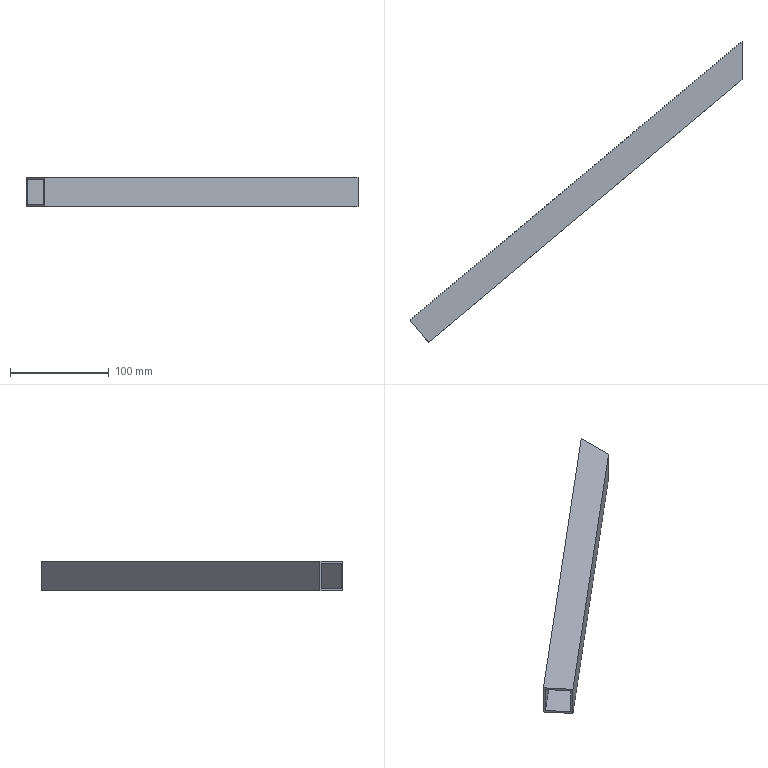Part | NX | features solid 2 | 1 solid | 10 faces | box 337.06 x 305.808 x 30 mm | volume 95741 mm3 | plane 10
STEP:
#1=CARTESIAN_POINT('',(30.,-60.,-105.));
#2=VERTEX_POINT('',#1);
#3=CARTESIAN_POINT('',(30.,-60.,-75.));
#4=VERTEX_POINT('',#3);
#5=CARTESIAN_POINT('',(30.,-60.,-105.));
#6=DIRECTION('',(0.,0.,1.));
#7=VECTOR('',#6,1000.);
#8=LINE('',#5,#7);
#9=EDGE_CURVE('',#2,#4,#8,.T.);
#10=ORIENTED_EDGE('',*,*,#9,.F.);
#11=CARTESIAN_POINT('',(-307.06,-342.827,-105.));
#12=VERTEX_POINT('',#11);
#13=CARTESIAN_POINT('',(-123.209,-188.558,-105.));
#14=DIRECTION('',(0.766,0.6428,0.));
#15=VECTOR('',#14,1000.);
#16=LINE('',#13,#15);
#17=EDGE_CURVE('',#12,#2,#16,.T.);
#18=ORIENTED_EDGE('',*,*,#17,.F.);
#19=CARTESIAN_POINT('',(-307.06,-342.827,-75.));
#20=VERTEX_POINT('',#19);
#21=CARTESIAN_POINT('',(-307.06,-342.827,-105.));
#22=DIRECTION('',(0.,0.,-1.));
#23=VECTOR('',#22,1000.);
#24=LINE('',#21,#23);
#25=EDGE_CURVE('',#12,#20,#24,.F.);
#26=ORIENTED_EDGE('',*,*,#25,.T.);
#27=CARTESIAN_POINT('',(-123.209,-188.558,-75.));
#28=DIRECTION('',(0.766,0.6428,0.));
#29=VECTOR('',#28,1000.);
#30=LINE('',#27,#29);
#31=EDGE_CURVE('',#20,#4,#30,.T.);
#32=ORIENTED_EDGE('',*,*,#31,.T.);
#33=EDGE_LOOP('',(#10,#18,#26,#32));
#34=FACE_BOUND('',#33,.T.);
#35=CARTESIAN_POINT('',(-123.209,-188.558,-105.));
#36=DIRECTION('',(-0.6428,0.766,0.));
#37=DIRECTION('',(0.,0.,1.));
#38=AXIS2_PLACEMENT_3D('',#35,#36,#37);
#39=PLANE('',#38);
#40=ADVANCED_FACE('',(#34),#39,.T.);
#41=CARTESIAN_POINT('',(30.,-99.162,-75.));
#42=VERTEX_POINT('',#41);
#43=CARTESIAN_POINT('',(30.,-188.558,-75.));
#44=DIRECTION('',(0.,-1.,0.));
#45=VECTOR('',#44,1000.);
#46=LINE('',#43,#45);
#47=EDGE_CURVE('',#4,#42,#46,.T.);
#48=ORIENTED_EDGE('',*,*,#47,.F.);
#49=ORIENTED_EDGE('',*,*,#31,.F.);
#50=CARTESIAN_POINT('',(-287.776,-365.808,-75.));
#51=VERTEX_POINT('',#50);
#52=CARTESIAN_POINT('',(-307.06,-342.827,-75.));
#53=DIRECTION('',(-0.6428,0.766,0.));
#54=VECTOR('',#53,1000.);
#55=LINE('',#52,#54);
#56=EDGE_CURVE('',#20,#51,#55,.F.);
#57=ORIENTED_EDGE('',*,*,#56,.T.);
#58=CARTESIAN_POINT('',(-103.925,-211.539,-75.));
#59=DIRECTION('',(0.766,0.6428,0.));
#60=VECTOR('',#59,1000.);
#61=LINE('',#58,#60);
#62=EDGE_CURVE('',#51,#42,#61,.T.);
#63=ORIENTED_EDGE('',*,*,#62,.T.);
#64=EDGE_LOOP('',(#48,#49,#57,#63));
#65=FACE_BOUND('',#64,.T.);
#66=CARTESIAN_POINT('',(-123.209,-188.558,-75.));
#67=DIRECTION('',(0.,0.,1.));
#68=DIRECTION('',(0.6428,-0.766,0.));
#69=AXIS2_PLACEMENT_3D('',#66,#67,#68);
#70=PLANE('',#69);
#71=ADVANCED_FACE('',(#65),#70,.T.);
#72=CARTESIAN_POINT('',(-287.776,-365.808,-105.));
#73=VERTEX_POINT('',#72);
#74=CARTESIAN_POINT('',(30.,-99.162,-105.));
#75=VERTEX_POINT('',#74);
#76=CARTESIAN_POINT('',(-103.925,-211.539,-105.));
#77=DIRECTION('',(0.766,0.6428,0.));
#78=VECTOR('',#77,1000.);
#79=LINE('',#76,#78);
#80=EDGE_CURVE('',#73,#75,#79,.T.);
#81=ORIENTED_EDGE('',*,*,#80,.T.);
#82=CARTESIAN_POINT('',(30.,-99.162,-105.));
#83=DIRECTION('',(0.,0.,1.));
#84=VECTOR('',#83,1000.);
#85=LINE('',#82,#84);
#86=EDGE_CURVE('',#75,#42,#85,.T.);
#87=ORIENTED_EDGE('',*,*,#86,.T.);
#88=ORIENTED_EDGE('',*,*,#62,.F.);
#89=CARTESIAN_POINT('',(-287.776,-365.808,-105.));
#90=DIRECTION('',(0.,0.,-1.));
#91=VECTOR('',#90,1000.);
#92=LINE('',#89,#91);
#93=EDGE_CURVE('',#73,#51,#92,.F.);
#94=ORIENTED_EDGE('',*,*,#93,.F.);
#95=EDGE_LOOP('',(#81,#87,#88,#94));
#96=FACE_BOUND('',#95,.T.);
#97=CARTESIAN_POINT('',(-103.925,-211.539,-105.));
#98=DIRECTION('',(-0.6428,0.766,0.));
#99=DIRECTION('',(0.,0.,1.));
#100=AXIS2_PLACEMENT_3D('',#97,#98,#99);
#101=PLANE('',#100);
#102=ADVANCED_FACE('',(#96),#101,.F.);
#103=ORIENTED_EDGE('',*,*,#17,.T.);
#104=CARTESIAN_POINT('',(30.,-188.558,-105.));
#105=DIRECTION('',(0.,-1.,0.));
#106=VECTOR('',#105,1000.);
#107=LINE('',#104,#106);
#108=EDGE_CURVE('',#2,#75,#107,.T.);
#109=ORIENTED_EDGE('',*,*,#108,.T.);
#110=ORIENTED_EDGE('',*,*,#80,.F.);
#111=CARTESIAN_POINT('',(-307.06,-342.827,-105.));
#112=DIRECTION('',(-0.6428,0.766,0.));
#113=VECTOR('',#112,1000.);
#114=LINE('',#111,#113);
#115=EDGE_CURVE('',#12,#73,#114,.F.);
#116=ORIENTED_EDGE('',*,*,#115,.F.);
#117=EDGE_LOOP('',(#103,#109,#110,#116));
#118=FACE_BOUND('',#117,.T.);
#119=CARTESIAN_POINT('',(-123.209,-188.558,-105.));
#120=DIRECTION('',(0.,0.,1.));
#121=DIRECTION('',(0.6428,-0.766,0.));
#122=AXIS2_PLACEMENT_3D('',#119,#120,#121);
#123=PLANE('',#122);
#124=ADVANCED_FACE('',(#118),#123,.F.);
#125=ORIENTED_EDGE('',*,*,#115,.T.);
#126=ORIENTED_EDGE('',*,*,#93,.T.);
#127=ORIENTED_EDGE('',*,*,#56,.F.);
#128=ORIENTED_EDGE('',*,*,#25,.F.);
#129=EDGE_LOOP('',(#125,#126,#127,#128));
#130=FACE_BOUND('',#129,.T.);
#131=CARTESIAN_POINT('',(-305.774,-344.359,-103.));
#132=VERTEX_POINT('',#131);
#133=CARTESIAN_POINT('',(-289.062,-364.276,-103.));
#134=VERTEX_POINT('',#133);
#135=CARTESIAN_POINT('',(-307.06,-342.827,-103.));
#136=DIRECTION('',(-0.6428,0.766,0.));
#137=VECTOR('',#136,1000.);
#138=LINE('',#135,#137);
#139=EDGE_CURVE('',#132,#134,#138,.F.);
#140=ORIENTED_EDGE('',*,*,#139,.F.);
#141=CARTESIAN_POINT('',(-305.774,-344.359,-77.));
#142=VERTEX_POINT('',#141);
#143=CARTESIAN_POINT('',(-305.774,-344.359,-105.));
#144=DIRECTION('',(0.,0.,-1.));
#145=VECTOR('',#144,1000.);
#146=LINE('',#143,#145);
#147=EDGE_CURVE('',#132,#142,#146,.F.);
#148=ORIENTED_EDGE('',*,*,#147,.T.);
#149=CARTESIAN_POINT('',(-289.062,-364.276,-77.));
#150=VERTEX_POINT('',#149);
#151=CARTESIAN_POINT('',(-307.06,-342.827,-77.));
#152=DIRECTION('',(-0.6428,0.766,0.));
#153=VECTOR('',#152,1000.);
#154=LINE('',#151,#153);
#155=EDGE_CURVE('',#142,#150,#154,.F.);
#156=ORIENTED_EDGE('',*,*,#155,.T.);
#157=CARTESIAN_POINT('',(-289.062,-364.276,-105.));
#158=DIRECTION('',(0.,0.,-1.));
#159=VECTOR('',#158,1000.);
#160=LINE('',#157,#159);
#161=EDGE_CURVE('',#134,#150,#160,.F.);
#162=ORIENTED_EDGE('',*,*,#161,.F.);
#163=EDGE_LOOP('',(#140,#148,#156,#162));
#164=FACE_BOUND('',#163,.T.);
#165=CARTESIAN_POINT('',(-307.06,-342.827,-105.));
#166=DIRECTION('',(-0.766,-0.6428,0.));
#167=DIRECTION('',(0.,0.,1.));
#168=AXIS2_PLACEMENT_3D('',#165,#166,#167);
#169=PLANE('',#168);
#170=ADVANCED_FACE('',(#130,#164),#169,.T.);
#171=CARTESIAN_POINT('',(30.,-62.611,-103.));
#172=VERTEX_POINT('',#171);
#173=CARTESIAN_POINT('',(-121.923,-190.09,-103.));
#174=DIRECTION('',(0.766,0.6428,0.));
#175=VECTOR('',#174,1000.);
#176=LINE('',#173,#175);
#177=EDGE_CURVE('',#132,#172,#176,.T.);
#178=ORIENTED_EDGE('',*,*,#177,.T.);
#179=CARTESIAN_POINT('',(30.,-62.611,-77.));
#180=VERTEX_POINT('',#179);
#181=CARTESIAN_POINT('',(30.,-62.611,-105.));
#182=DIRECTION('',(0.,0.,1.));
#183=VECTOR('',#182,1000.);
#184=LINE('',#181,#183);
#185=EDGE_CURVE('',#172,#180,#184,.T.);
#186=ORIENTED_EDGE('',*,*,#185,.T.);
#187=CARTESIAN_POINT('',(-121.923,-190.09,-77.));
#188=DIRECTION('',(0.766,0.6428,0.));
#189=VECTOR('',#188,1000.);
#190=LINE('',#187,#189);
#191=EDGE_CURVE('',#142,#180,#190,.T.);
#192=ORIENTED_EDGE('',*,*,#191,.F.);
#193=ORIENTED_EDGE('',*,*,#147,.F.);
#194=EDGE_LOOP('',(#178,#186,#192,#193));
#195=FACE_BOUND('',#194,.T.);
#196=CARTESIAN_POINT('',(-121.923,-190.09,-105.));
#197=DIRECTION('',(-0.6428,0.766,0.));
#198=DIRECTION('',(0.,0.,1.));
#199=AXIS2_PLACEMENT_3D('',#196,#197,#198);
#200=PLANE('',#199);
#201=ADVANCED_FACE('',(#195),#200,.F.);
#202=ORIENTED_EDGE('',*,*,#191,.T.);
#203=CARTESIAN_POINT('',(30.,-96.551,-77.));
#204=VERTEX_POINT('',#203);
#205=CARTESIAN_POINT('',(30.,-188.558,-77.));
#206=DIRECTION('',(0.,-1.,0.));
#207=VECTOR('',#206,1000.);
#208=LINE('',#205,#207);
#209=EDGE_CURVE('',#180,#204,#208,.T.);
#210=ORIENTED_EDGE('',*,*,#209,.T.);
#211=CARTESIAN_POINT('',(-105.211,-210.007,-77.));
#212=DIRECTION('',(0.766,0.6428,0.));
#213=VECTOR('',#212,1000.);
#214=LINE('',#211,#213);
#215=EDGE_CURVE('',#150,#204,#214,.T.);
#216=ORIENTED_EDGE('',*,*,#215,.F.);
#217=ORIENTED_EDGE('',*,*,#155,.F.);
#218=EDGE_LOOP('',(#202,#210,#216,#217));
#219=FACE_BOUND('',#218,.T.);
#220=CARTESIAN_POINT('',(-123.209,-188.558,-77.));
#221=DIRECTION('',(0.,0.,1.));
#222=DIRECTION('',(0.6428,-0.766,0.));
#223=AXIS2_PLACEMENT_3D('',#220,#221,#222);
#224=PLANE('',#223);
#225=ADVANCED_FACE('',(#219),#224,.F.);
#226=CARTESIAN_POINT('',(30.,-96.551,-103.));
#227=VERTEX_POINT('',#226);
#228=CARTESIAN_POINT('',(30.,-96.551,-105.));
#229=DIRECTION('',(0.,0.,1.));
#230=VECTOR('',#229,1000.);
#231=LINE('',#228,#230);
#232=EDGE_CURVE('',#227,#204,#231,.T.);
#233=ORIENTED_EDGE('',*,*,#232,.F.);
#234=CARTESIAN_POINT('',(-105.211,-210.007,-103.));
#235=DIRECTION('',(0.766,0.6428,0.));
#236=VECTOR('',#235,1000.);
#237=LINE('',#234,#236);
#238=EDGE_CURVE('',#134,#227,#237,.T.);
#239=ORIENTED_EDGE('',*,*,#238,.F.);
#240=ORIENTED_EDGE('',*,*,#161,.T.);
#241=ORIENTED_EDGE('',*,*,#215,.T.);
#242=EDGE_LOOP('',(#233,#239,#240,#241));
#243=FACE_BOUND('',#242,.T.);
#244=CARTESIAN_POINT('',(-105.211,-210.007,-105.));
#245=DIRECTION('',(-0.6428,0.766,0.));
#246=DIRECTION('',(0.,0.,1.));
#247=AXIS2_PLACEMENT_3D('',#244,#245,#246);
#248=PLANE('',#247);
#249=ADVANCED_FACE('',(#243),#248,.T.);
#250=CARTESIAN_POINT('',(30.,-188.558,-103.));
#251=DIRECTION('',(0.,-1.,0.));
#252=VECTOR('',#251,1000.);
#253=LINE('',#250,#252);
#254=EDGE_CURVE('',#172,#227,#253,.T.);
#255=ORIENTED_EDGE('',*,*,#254,.F.);
#256=ORIENTED_EDGE('',*,*,#177,.F.);
#257=ORIENTED_EDGE('',*,*,#139,.T.);
#258=ORIENTED_EDGE('',*,*,#238,.T.);
#259=EDGE_LOOP('',(#255,#256,#257,#258));
#260=FACE_BOUND('',#259,.T.);
#261=CARTESIAN_POINT('',(-123.209,-188.558,-103.));
#262=DIRECTION('',(0.,0.,1.));
#263=DIRECTION('',(0.6428,-0.766,0.));
#264=AXIS2_PLACEMENT_3D('',#261,#262,#263);
#265=PLANE('',#264);
#266=ADVANCED_FACE('',(#260),#265,.T.);
#267=ORIENTED_EDGE('',*,*,#254,.T.);
#268=ORIENTED_EDGE('',*,*,#232,.T.);
#269=ORIENTED_EDGE('',*,*,#209,.F.);
#270=ORIENTED_EDGE('',*,*,#185,.F.);
#271=EDGE_LOOP('',(#267,#268,#269,#270));
#272=FACE_BOUND('',#271,.T.);
#273=ORIENTED_EDGE('',*,*,#9,.T.);
#274=ORIENTED_EDGE('',*,*,#47,.T.);
#275=ORIENTED_EDGE('',*,*,#86,.F.);
#276=ORIENTED_EDGE('',*,*,#108,.F.);
#277=EDGE_LOOP('',(#273,#274,#275,#276));
#278=FACE_BOUND('',#277,.T.);
#279=CARTESIAN_POINT('',(30.,115.,-45.));
#280=DIRECTION('',(-1.,0.,0.));
#281=DIRECTION('',(0.,-1.,0.));
#282=AXIS2_PLACEMENT_3D('',#279,#280,#281);
#283=PLANE('',#282);
#284=ADVANCED_FACE('',(#272,#278),#283,.F.);
#285=CLOSED_SHELL('',(#40,#71,#102,#124,#170,#201,#225,#249,#266,#284));
#286=MANIFOLD_SOLID_BREP('',#285);
#287=(LENGTH_UNIT()NAMED_UNIT(*)SI_UNIT(.MILLI.,.METRE.));
#288=UNCERTAINTY_MEASURE_WITH_UNIT(LENGTH_MEASURE(0.00001),#287,'','');
#289=(NAMED_UNIT(*)PLANE_ANGLE_UNIT()SI_UNIT($,.RADIAN.));
#290=(NAMED_UNIT(*)SI_UNIT($,.STERADIAN.)SOLID_ANGLE_UNIT());
#291=(GEOMETRIC_REPRESENTATION_CONTEXT(3)GLOBAL_UNCERTAINTY_ASSIGNED_CONTEXT((#288))GLOBAL_UNIT_ASSIGNED_CONTEXT((#287,#289,#290))REPRESENTATION_CONTEXT('',''));
#292=ADVANCED_BREP_SHAPE_REPRESENTATION('',(#286),#291);